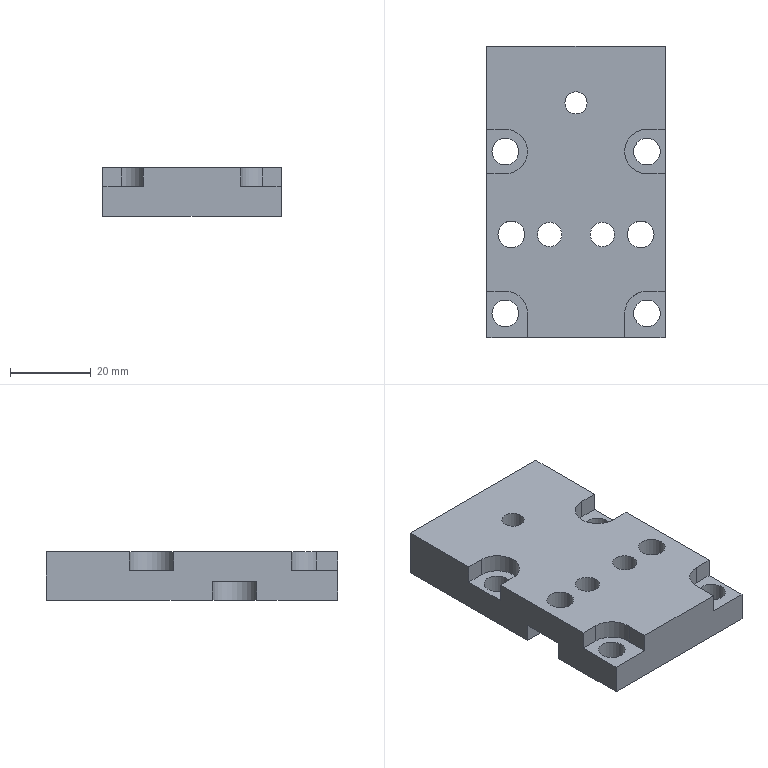Part | NX | features BREP 1 | 1 solid | 41 faces | box 44 x 72 x 12 mm | volume 32304 mm3 | plane 25 | cylinder 16 | commonest cylinder face diameters 6.6 x6 11 x6 6 x2 5.5 x1 10 x1
STEP:
#1=CARTESIAN_POINT('',(-22.,36.,0.));
#2=VERTEX_POINT('',#1);
#3=CARTESIAN_POINT('',(-22.,-5.,0.));
#4=VERTEX_POINT('',#3);
#5=CARTESIAN_POINT('',(-22.,0.,0.));
#6=DIRECTION('',(0.,-1.,0.));
#7=VECTOR('',#6,1000.);
#8=LINE('',#5,#7);
#9=EDGE_CURVE('',#2,#4,#8,.T.);
#10=ORIENTED_EDGE('',*,*,#9,.F.);
#11=CARTESIAN_POINT('',(22.,36.,0.));
#12=VERTEX_POINT('',#11);
#13=CARTESIAN_POINT('',(0.,36.,0.));
#14=DIRECTION('',(-1.,0.,0.));
#15=VECTOR('',#14,1000.);
#16=LINE('',#13,#15);
#17=EDGE_CURVE('',#12,#2,#16,.T.);
#18=ORIENTED_EDGE('',*,*,#17,.F.);
#19=CARTESIAN_POINT('',(22.,-5.,0.));
#20=VERTEX_POINT('',#19);
#21=CARTESIAN_POINT('',(22.,0.,0.));
#22=DIRECTION('',(0.,1.,0.));
#23=VECTOR('',#22,1000.);
#24=LINE('',#21,#23);
#25=EDGE_CURVE('',#20,#12,#24,.T.);
#26=ORIENTED_EDGE('',*,*,#25,.F.);
#27=CARTESIAN_POINT('',(16.,-5.,0.));
#28=VERTEX_POINT('',#27);
#29=CARTESIAN_POINT('',(0.,-5.,0.));
#30=DIRECTION('',(1.,0.,0.));
#31=VECTOR('',#30,1000.);
#32=LINE('',#29,#31);
#33=EDGE_CURVE('',#28,#20,#32,.T.);
#34=ORIENTED_EDGE('',*,*,#33,.F.);
#35=CARTESIAN_POINT('',(16.,-16.,0.));
#36=VERTEX_POINT('',#35);
#37=CARTESIAN_POINT('',(16.,-10.5,0.));
#38=DIRECTION('',(0.,0.,-1.));
#39=DIRECTION('',(-1.,0.,0.));
#40=AXIS2_PLACEMENT_3D('',#37,#38,#39);
#41=CIRCLE('',#40,5.5);
#42=EDGE_CURVE('',#36,#28,#41,.T.);
#43=ORIENTED_EDGE('',*,*,#42,.F.);
#44=CARTESIAN_POINT('',(22.,-16.,0.));
#45=VERTEX_POINT('',#44);
#46=CARTESIAN_POINT('',(0.,-16.,0.));
#47=DIRECTION('',(-1.,0.,0.));
#48=VECTOR('',#47,1000.);
#49=LINE('',#46,#48);
#50=EDGE_CURVE('',#45,#36,#49,.T.);
#51=ORIENTED_EDGE('',*,*,#50,.F.);
#52=CARTESIAN_POINT('',(22.,-36.,0.));
#53=VERTEX_POINT('',#52);
#54=CARTESIAN_POINT('',(22.,0.,0.));
#55=DIRECTION('',(0.,1.,0.));
#56=VECTOR('',#55,1000.);
#57=LINE('',#54,#56);
#58=EDGE_CURVE('',#53,#45,#57,.T.);
#59=ORIENTED_EDGE('',*,*,#58,.F.);
#60=CARTESIAN_POINT('',(-22.,-36.,0.));
#61=VERTEX_POINT('',#60);
#62=CARTESIAN_POINT('',(0.,-36.,0.));
#63=DIRECTION('',(1.,0.,0.));
#64=VECTOR('',#63,1000.);
#65=LINE('',#62,#64);
#66=EDGE_CURVE('',#61,#53,#65,.T.);
#67=ORIENTED_EDGE('',*,*,#66,.F.);
#68=CARTESIAN_POINT('',(-22.,-16.,0.));
#69=VERTEX_POINT('',#68);
#70=CARTESIAN_POINT('',(-22.,0.,0.));
#71=DIRECTION('',(0.,-1.,0.));
#72=VECTOR('',#71,1000.);
#73=LINE('',#70,#72);
#74=EDGE_CURVE('',#69,#61,#73,.T.);
#75=ORIENTED_EDGE('',*,*,#74,.F.);
#76=CARTESIAN_POINT('',(-16.,-16.,0.));
#77=VERTEX_POINT('',#76);
#78=CARTESIAN_POINT('',(0.,-16.,0.));
#79=DIRECTION('',(-1.,0.,0.));
#80=VECTOR('',#79,1000.);
#81=LINE('',#78,#80);
#82=EDGE_CURVE('',#77,#69,#81,.T.);
#83=ORIENTED_EDGE('',*,*,#82,.F.);
#84=CARTESIAN_POINT('',(-16.,-5.,0.));
#85=VERTEX_POINT('',#84);
#86=CARTESIAN_POINT('',(-16.,-10.5,0.));
#87=DIRECTION('',(0.,0.,-1.));
#88=DIRECTION('',(-1.,0.,0.));
#89=AXIS2_PLACEMENT_3D('',#86,#87,#88);
#90=CIRCLE('',#89,5.5);
#91=EDGE_CURVE('',#85,#77,#90,.T.);
#92=ORIENTED_EDGE('',*,*,#91,.F.);
#93=CARTESIAN_POINT('',(0.,-5.,0.));
#94=DIRECTION('',(1.,0.,0.));
#95=VECTOR('',#94,1000.);
#96=LINE('',#93,#95);
#97=EDGE_CURVE('',#4,#85,#96,.T.);
#98=ORIENTED_EDGE('',*,*,#97,.F.);
#99=EDGE_LOOP('',(#10,#18,#26,#34,#43,#51,#59,#67,#75,#83,#92,#98));
#100=FACE_BOUND('',#99,.T.);
#101=CARTESIAN_POINT('',(-3.5,-10.5,0.));
#102=VERTEX_POINT('',#101);
#103=CARTESIAN_POINT('',(-6.5,-10.5,0.));
#104=DIRECTION('',(0.,0.,-1.));
#105=DIRECTION('',(1.,0.,0.));
#106=AXIS2_PLACEMENT_3D('',#103,#104,#105);
#107=CIRCLE('',#106,3.);
#108=EDGE_CURVE('',#102,#102,#107,.T.);
#109=ORIENTED_EDGE('',*,*,#108,.F.);
#110=EDGE_LOOP('',(#109));
#111=FACE_BOUND('',#110,.T.);
#112=CARTESIAN_POINT('',(9.5,-10.5,0.));
#113=VERTEX_POINT('',#112);
#114=CARTESIAN_POINT('',(6.5,-10.5,0.));
#115=DIRECTION('',(0.,0.,-1.));
#116=DIRECTION('',(1.,0.,0.));
#117=AXIS2_PLACEMENT_3D('',#114,#115,#116);
#118=CIRCLE('',#117,3.);
#119=EDGE_CURVE('',#113,#113,#118,.T.);
#120=ORIENTED_EDGE('',*,*,#119,.F.);
#121=EDGE_LOOP('',(#120));
#122=FACE_BOUND('',#121,.T.);
#123=CARTESIAN_POINT('',(20.825,-30.,0.));
#124=VERTEX_POINT('',#123);
#125=CARTESIAN_POINT('',(17.525,-30.,0.));
#126=DIRECTION('',(0.,0.,-1.));
#127=DIRECTION('',(1.,0.,0.));
#128=AXIS2_PLACEMENT_3D('',#125,#126,#127);
#129=CIRCLE('',#128,3.3);
#130=EDGE_CURVE('',#124,#124,#129,.T.);
#131=ORIENTED_EDGE('',*,*,#130,.F.);
#132=EDGE_LOOP('',(#131));
#133=FACE_BOUND('',#132,.T.);
#134=CARTESIAN_POINT('',(-14.175,-30.,0.));
#135=VERTEX_POINT('',#134);
#136=CARTESIAN_POINT('',(-17.475,-30.,0.));
#137=DIRECTION('',(0.,0.,-1.));
#138=DIRECTION('',(1.,0.,0.));
#139=AXIS2_PLACEMENT_3D('',#136,#137,#138);
#140=CIRCLE('',#139,3.3);
#141=EDGE_CURVE('',#135,#135,#140,.T.);
#142=ORIENTED_EDGE('',*,*,#141,.F.);
#143=EDGE_LOOP('',(#142));
#144=FACE_BOUND('',#143,.T.);
#145=CARTESIAN_POINT('',(-14.175,10.,0.));
#146=VERTEX_POINT('',#145);
#147=CARTESIAN_POINT('',(-17.475,10.,0.));
#148=DIRECTION('',(0.,0.,-1.));
#149=DIRECTION('',(1.,0.,0.));
#150=AXIS2_PLACEMENT_3D('',#147,#148,#149);
#151=CIRCLE('',#150,3.3);
#152=EDGE_CURVE('',#146,#146,#151,.T.);
#153=ORIENTED_EDGE('',*,*,#152,.F.);
#154=EDGE_LOOP('',(#153));
#155=FACE_BOUND('',#154,.T.);
#156=CARTESIAN_POINT('',(20.825,10.,0.));
#157=VERTEX_POINT('',#156);
#158=CARTESIAN_POINT('',(17.525,10.,0.));
#159=DIRECTION('',(0.,0.,-1.));
#160=DIRECTION('',(1.,0.,0.));
#161=AXIS2_PLACEMENT_3D('',#158,#159,#160);
#162=CIRCLE('',#161,3.3);
#163=EDGE_CURVE('',#157,#157,#162,.T.);
#164=ORIENTED_EDGE('',*,*,#163,.F.);
#165=EDGE_LOOP('',(#164));
#166=FACE_BOUND('',#165,.T.);
#167=CARTESIAN_POINT('',(-5.,22.,0.));
#168=VERTEX_POINT('',#167);
#169=CARTESIAN_POINT('',(0.,22.,0.));
#170=DIRECTION('',(0.,0.,-1.));
#171=DIRECTION('',(-1.,0.,0.));
#172=AXIS2_PLACEMENT_3D('',#169,#170,#171);
#173=CIRCLE('',#172,5.);
#174=EDGE_CURVE('',#168,#168,#173,.T.);
#175=ORIENTED_EDGE('',*,*,#174,.F.);
#176=EDGE_LOOP('',(#175));
#177=FACE_BOUND('',#176,.T.);
#178=CARTESIAN_POINT('',(0.,0.,0.));
#179=DIRECTION('',(0.,0.,1.));
#180=DIRECTION('',(-1.,0.,0.));
#181=AXIS2_PLACEMENT_3D('',#178,#179,#180);
#182=PLANE('',#181);
#183=ADVANCED_FACE('',(#100,#111,#122,#133,#144,#155,#166,#177),#182,.F.);
#184=ORIENTED_EDGE('',*,*,#97,.T.);
#185=CARTESIAN_POINT('',(-16.,-5.,4.6));
#186=VERTEX_POINT('',#185);
#187=CARTESIAN_POINT('',(-16.,-5.,17.13));
#188=DIRECTION('',(0.,0.,1.));
#189=VECTOR('',#188,1000.);
#190=LINE('',#187,#189);
#191=EDGE_CURVE('',#85,#186,#190,.T.);
#192=ORIENTED_EDGE('',*,*,#191,.T.);
#193=CARTESIAN_POINT('',(-22.,-5.,4.6));
#194=VERTEX_POINT('',#193);
#195=CARTESIAN_POINT('',(-16.,-5.,4.6));
#196=DIRECTION('',(-1.,0.,0.));
#197=VECTOR('',#196,1000.);
#198=LINE('',#195,#197);
#199=EDGE_CURVE('',#186,#194,#198,.T.);
#200=ORIENTED_EDGE('',*,*,#199,.T.);
#201=CARTESIAN_POINT('',(-22.,-5.,17.13));
#202=DIRECTION('',(0.,0.,-1.));
#203=VECTOR('',#202,1000.);
#204=LINE('',#201,#203);
#205=EDGE_CURVE('',#194,#4,#204,.T.);
#206=ORIENTED_EDGE('',*,*,#205,.T.);
#207=EDGE_LOOP('',(#184,#192,#200,#206));
#208=FACE_BOUND('',#207,.T.);
#209=CARTESIAN_POINT('',(-16.,-5.,17.13));
#210=DIRECTION('',(0.,-1.,0.));
#211=DIRECTION('',(-1.,0.,0.));
#212=AXIS2_PLACEMENT_3D('',#209,#210,#211);
#213=PLANE('',#212);
#214=ADVANCED_FACE('',(#208),#213,.T.);
#215=CARTESIAN_POINT('',(-22.,-16.,4.6));
#216=VERTEX_POINT('',#215);
#217=CARTESIAN_POINT('',(-22.,36.,4.6));
#218=DIRECTION('',(0.,1.,0.));
#219=VECTOR('',#218,1000.);
#220=LINE('',#217,#219);
#221=EDGE_CURVE('',#216,#194,#220,.T.);
#222=ORIENTED_EDGE('',*,*,#221,.F.);
#223=CARTESIAN_POINT('',(-22.,-16.,12.));
#224=DIRECTION('',(0.,0.,1.));
#225=VECTOR('',#224,1000.);
#226=LINE('',#223,#225);
#227=EDGE_CURVE('',#69,#216,#226,.T.);
#228=ORIENTED_EDGE('',*,*,#227,.F.);
#229=ORIENTED_EDGE('',*,*,#74,.T.);
#230=CARTESIAN_POINT('',(-22.,-36.,7.4));
#231=VERTEX_POINT('',#230);
#232=CARTESIAN_POINT('',(-22.,-36.,12.));
#233=DIRECTION('',(0.,0.,-1.));
#234=VECTOR('',#233,1000.);
#235=LINE('',#232,#234);
#236=EDGE_CURVE('',#231,#61,#235,.T.);
#237=ORIENTED_EDGE('',*,*,#236,.F.);
#238=CARTESIAN_POINT('',(-22.,-24.5,7.4));
#239=VERTEX_POINT('',#238);
#240=CARTESIAN_POINT('',(-22.,36.,7.4));
#241=DIRECTION('',(0.,-1.,0.));
#242=VECTOR('',#241,1000.);
#243=LINE('',#240,#242);
#244=EDGE_CURVE('',#239,#231,#243,.T.);
#245=ORIENTED_EDGE('',*,*,#244,.F.);
#246=CARTESIAN_POINT('',(-22.,-24.5,12.));
#247=VERTEX_POINT('',#246);
#248=CARTESIAN_POINT('',(-22.,-24.5,12.));
#249=DIRECTION('',(0.,0.,-1.));
#250=VECTOR('',#249,1000.);
#251=LINE('',#248,#250);
#252=EDGE_CURVE('',#247,#239,#251,.T.);
#253=ORIENTED_EDGE('',*,*,#252,.F.);
#254=CARTESIAN_POINT('',(-22.,4.5,12.));
#255=VERTEX_POINT('',#254);
#256=CARTESIAN_POINT('',(-22.,36.,12.));
#257=DIRECTION('',(0.,-1.,0.));
#258=VECTOR('',#257,1000.);
#259=LINE('',#256,#258);
#260=EDGE_CURVE('',#255,#247,#259,.T.);
#261=ORIENTED_EDGE('',*,*,#260,.F.);
#262=CARTESIAN_POINT('',(-22.,4.5,7.4));
#263=VERTEX_POINT('',#262);
#264=CARTESIAN_POINT('',(-22.,4.5,12.));
#265=DIRECTION('',(0.,0.,1.));
#266=VECTOR('',#265,1000.);
#267=LINE('',#264,#266);
#268=EDGE_CURVE('',#263,#255,#267,.T.);
#269=ORIENTED_EDGE('',*,*,#268,.F.);
#270=CARTESIAN_POINT('',(-22.,15.5,7.4));
#271=VERTEX_POINT('',#270);
#272=CARTESIAN_POINT('',(-22.,36.,7.4));
#273=DIRECTION('',(0.,-1.,0.));
#274=VECTOR('',#273,1000.);
#275=LINE('',#272,#274);
#276=EDGE_CURVE('',#271,#263,#275,.T.);
#277=ORIENTED_EDGE('',*,*,#276,.F.);
#278=CARTESIAN_POINT('',(-22.,15.5,12.));
#279=VERTEX_POINT('',#278);
#280=CARTESIAN_POINT('',(-22.,15.5,12.));
#281=DIRECTION('',(0.,0.,-1.));
#282=VECTOR('',#281,1000.);
#283=LINE('',#280,#282);
#284=EDGE_CURVE('',#279,#271,#283,.T.);
#285=ORIENTED_EDGE('',*,*,#284,.F.);
#286=CARTESIAN_POINT('',(-22.,36.,12.));
#287=VERTEX_POINT('',#286);
#288=CARTESIAN_POINT('',(-22.,36.,12.));
#289=DIRECTION('',(0.,-1.,0.));
#290=VECTOR('',#289,1000.);
#291=LINE('',#288,#290);
#292=EDGE_CURVE('',#287,#279,#291,.T.);
#293=ORIENTED_EDGE('',*,*,#292,.F.);
#294=CARTESIAN_POINT('',(-22.,36.,12.));
#295=DIRECTION('',(0.,0.,1.));
#296=VECTOR('',#295,1000.);
#297=LINE('',#294,#296);
#298=EDGE_CURVE('',#2,#287,#297,.T.);
#299=ORIENTED_EDGE('',*,*,#298,.F.);
#300=ORIENTED_EDGE('',*,*,#9,.T.);
#301=ORIENTED_EDGE('',*,*,#205,.F.);
#302=EDGE_LOOP('',(#222,#228,#229,#237,#245,#253,#261,#269,#277,#285,#293,#299,#300,#301));
#303=FACE_BOUND('',#302,.T.);
#304=CARTESIAN_POINT('',(-22.,36.,12.));
#305=DIRECTION('',(1.,0.,0.));
#306=DIRECTION('',(0.,-1.,0.));
#307=AXIS2_PLACEMENT_3D('',#304,#305,#306);
#308=PLANE('',#307);
#309=ADVANCED_FACE('',(#303),#308,.F.);
#310=ORIENTED_EDGE('',*,*,#298,.T.);
#311=CARTESIAN_POINT('',(22.,36.,12.));
#312=VERTEX_POINT('',#311);
#313=CARTESIAN_POINT('',(-22.,36.,12.));
#314=DIRECTION('',(-1.,0.,0.));
#315=VECTOR('',#314,1000.);
#316=LINE('',#313,#315);
#317=EDGE_CURVE('',#312,#287,#316,.T.);
#318=ORIENTED_EDGE('',*,*,#317,.F.);
#319=CARTESIAN_POINT('',(22.,36.,12.));
#320=DIRECTION('',(0.,0.,1.));
#321=VECTOR('',#320,1000.);
#322=LINE('',#319,#321);
#323=EDGE_CURVE('',#12,#312,#322,.T.);
#324=ORIENTED_EDGE('',*,*,#323,.F.);
#325=ORIENTED_EDGE('',*,*,#17,.T.);
#326=EDGE_LOOP('',(#310,#318,#324,#325));
#327=FACE_BOUND('',#326,.T.);
#328=CARTESIAN_POINT('',(-22.,36.,12.));
#329=DIRECTION('',(0.,-1.,0.));
#330=DIRECTION('',(0.,0.,1.));
#331=AXIS2_PLACEMENT_3D('',#328,#329,#330);
#332=PLANE('',#331);
#333=ADVANCED_FACE('',(#327),#332,.F.);
#334=CARTESIAN_POINT('',(22.,-5.,4.6));
#335=VERTEX_POINT('',#334);
#336=CARTESIAN_POINT('',(22.,-5.,12.));
#337=DIRECTION('',(0.,0.,1.));
#338=VECTOR('',#337,1000.);
#339=LINE('',#336,#338);
#340=EDGE_CURVE('',#20,#335,#339,.T.);
#341=ORIENTED_EDGE('',*,*,#340,.F.);
#342=ORIENTED_EDGE('',*,*,#25,.T.);
#343=ORIENTED_EDGE('',*,*,#323,.T.);
#344=CARTESIAN_POINT('',(22.,15.5,12.));
#345=VERTEX_POINT('',#344);
#346=CARTESIAN_POINT('',(22.,36.,12.));
#347=DIRECTION('',(0.,1.,0.));
#348=VECTOR('',#347,1000.);
#349=LINE('',#346,#348);
#350=EDGE_CURVE('',#345,#312,#349,.T.);
#351=ORIENTED_EDGE('',*,*,#350,.F.);
#352=CARTESIAN_POINT('',(22.,15.5,7.4));
#353=VERTEX_POINT('',#352);
#354=CARTESIAN_POINT('',(22.,15.5,12.));
#355=DIRECTION('',(0.,0.,1.));
#356=VECTOR('',#355,1000.);
#357=LINE('',#354,#356);
#358=EDGE_CURVE('',#353,#345,#357,.T.);
#359=ORIENTED_EDGE('',*,*,#358,.F.);
#360=CARTESIAN_POINT('',(22.,4.5,7.4));
#361=VERTEX_POINT('',#360);
#362=CARTESIAN_POINT('',(22.,36.,7.4));
#363=DIRECTION('',(0.,1.,0.));
#364=VECTOR('',#363,1000.);
#365=LINE('',#362,#364);
#366=EDGE_CURVE('',#361,#353,#365,.T.);
#367=ORIENTED_EDGE('',*,*,#366,.F.);
#368=CARTESIAN_POINT('',(22.,4.5,12.));
#369=VERTEX_POINT('',#368);
#370=CARTESIAN_POINT('',(22.,4.5,12.));
#371=DIRECTION('',(0.,0.,-1.));
#372=VECTOR('',#371,1000.);
#373=LINE('',#370,#372);
#374=EDGE_CURVE('',#369,#361,#373,.T.);
#375=ORIENTED_EDGE('',*,*,#374,.F.);
#376=CARTESIAN_POINT('',(22.,-24.5,12.));
#377=VERTEX_POINT('',#376);
#378=CARTESIAN_POINT('',(22.,36.,12.));
#379=DIRECTION('',(0.,1.,0.));
#380=VECTOR('',#379,1000.);
#381=LINE('',#378,#380);
#382=EDGE_CURVE('',#377,#369,#381,.T.);
#383=ORIENTED_EDGE('',*,*,#382,.F.);
#384=CARTESIAN_POINT('',(22.,-24.5,7.4));
#385=VERTEX_POINT('',#384);
#386=CARTESIAN_POINT('',(22.,-24.5,12.));
#387=DIRECTION('',(0.,0.,1.));
#388=VECTOR('',#387,1000.);
#389=LINE('',#386,#388);
#390=EDGE_CURVE('',#385,#377,#389,.T.);
#391=ORIENTED_EDGE('',*,*,#390,.F.);
#392=CARTESIAN_POINT('',(22.,-36.,7.4));
#393=VERTEX_POINT('',#392);
#394=CARTESIAN_POINT('',(22.,36.,7.4));
#395=DIRECTION('',(0.,1.,0.));
#396=VECTOR('',#395,1000.);
#397=LINE('',#394,#396);
#398=EDGE_CURVE('',#393,#385,#397,.T.);
#399=ORIENTED_EDGE('',*,*,#398,.F.);
#400=CARTESIAN_POINT('',(22.,-36.,12.));
#401=DIRECTION('',(0.,0.,1.));
#402=VECTOR('',#401,1000.);
#403=LINE('',#400,#402);
#404=EDGE_CURVE('',#53,#393,#403,.T.);
#405=ORIENTED_EDGE('',*,*,#404,.F.);
#406=ORIENTED_EDGE('',*,*,#58,.T.);
#407=CARTESIAN_POINT('',(22.,-16.,4.6));
#408=VERTEX_POINT('',#407);
#409=CARTESIAN_POINT('',(22.,-16.,12.));
#410=DIRECTION('',(0.,0.,-1.));
#411=VECTOR('',#410,1000.);
#412=LINE('',#409,#411);
#413=EDGE_CURVE('',#408,#45,#412,.T.);
#414=ORIENTED_EDGE('',*,*,#413,.F.);
#415=CARTESIAN_POINT('',(22.,36.,4.6));
#416=DIRECTION('',(0.,-1.,0.));
#417=VECTOR('',#416,1000.);
#418=LINE('',#415,#417);
#419=EDGE_CURVE('',#335,#408,#418,.T.);
#420=ORIENTED_EDGE('',*,*,#419,.F.);
#421=EDGE_LOOP('',(#341,#342,#343,#351,#359,#367,#375,#383,#391,#399,#405,#406,#414,#420));
#422=FACE_BOUND('',#421,.T.);
#423=CARTESIAN_POINT('',(22.,36.,12.));
#424=DIRECTION('',(-1.,0.,0.));
#425=DIRECTION('',(0.,1.,0.));
#426=AXIS2_PLACEMENT_3D('',#423,#424,#425);
#427=PLANE('',#426);
#428=ADVANCED_FACE('',(#422),#427,.F.);
#429=ORIENTED_EDGE('',*,*,#33,.T.);
#430=ORIENTED_EDGE('',*,*,#340,.T.);
#431=CARTESIAN_POINT('',(16.,-5.,4.6));
#432=VERTEX_POINT('',#431);
#433=CARTESIAN_POINT('',(16.,-5.,4.6));
#434=DIRECTION('',(1.,0.,0.));
#435=VECTOR('',#434,1000.);
#436=LINE('',#433,#435);
#437=EDGE_CURVE('',#432,#335,#436,.T.);
#438=ORIENTED_EDGE('',*,*,#437,.F.);
#439=CARTESIAN_POINT('',(16.,-5.,17.13));
#440=DIRECTION('',(0.,0.,1.));
#441=VECTOR('',#440,1000.);
#442=LINE('',#439,#441);
#443=EDGE_CURVE('',#28,#432,#442,.T.);
#444=ORIENTED_EDGE('',*,*,#443,.F.);
#445=EDGE_LOOP('',(#429,#430,#438,#444));
#446=FACE_BOUND('',#445,.T.);
#447=CARTESIAN_POINT('',(16.,-5.,17.13));
#448=DIRECTION('',(0.,1.,0.));
#449=DIRECTION('',(1.,0.,0.));
#450=AXIS2_PLACEMENT_3D('',#447,#448,#449);
#451=PLANE('',#450);
#452=ADVANCED_FACE('',(#446),#451,.F.);
#453=CARTESIAN_POINT('',(16.,-16.,4.6));
#454=VERTEX_POINT('',#453);
#455=CARTESIAN_POINT('',(16.,-10.5,4.6));
#456=DIRECTION('',(0.,0.,-1.));
#457=DIRECTION('',(-1.,0.,0.));
#458=AXIS2_PLACEMENT_3D('',#455,#456,#457);
#459=CIRCLE('',#458,5.5);
#460=EDGE_CURVE('',#454,#432,#459,.T.);
#461=ORIENTED_EDGE('',*,*,#460,.F.);
#462=CARTESIAN_POINT('',(16.,-16.,0.));
#463=DIRECTION('',(0.,0.,1.));
#464=VECTOR('',#463,1000.);
#465=LINE('',#462,#464);
#466=EDGE_CURVE('',#36,#454,#465,.T.);
#467=ORIENTED_EDGE('',*,*,#466,.F.);
#468=ORIENTED_EDGE('',*,*,#42,.T.);
#469=ORIENTED_EDGE('',*,*,#443,.T.);
#470=EDGE_LOOP('',(#461,#467,#468,#469));
#471=FACE_BOUND('',#470,.T.);
#472=CARTESIAN_POINT('',(16.,-10.5,0.));
#473=DIRECTION('',(0.,0.,-1.));
#474=DIRECTION('',(1.,0.,0.));
#475=AXIS2_PLACEMENT_3D('',#472,#473,#474);
#476=CYLINDRICAL_SURFACE('',#475,5.5);
#477=ADVANCED_FACE('',(#471),#476,.F.);
#478=ORIENTED_EDGE('',*,*,#50,.T.);
#479=ORIENTED_EDGE('',*,*,#466,.T.);
#480=CARTESIAN_POINT('',(22.,-16.,4.6));
#481=DIRECTION('',(-1.,0.,0.));
#482=VECTOR('',#481,1000.);
#483=LINE('',#480,#482);
#484=EDGE_CURVE('',#408,#454,#483,.T.);
#485=ORIENTED_EDGE('',*,*,#484,.F.);
#486=ORIENTED_EDGE('',*,*,#413,.T.);
#487=EDGE_LOOP('',(#478,#479,#485,#486));
#488=FACE_BOUND('',#487,.T.);
#489=CARTESIAN_POINT('',(22.,-16.,17.13));
#490=DIRECTION('',(0.,-1.,0.));
#491=DIRECTION('',(-1.,0.,0.));
#492=AXIS2_PLACEMENT_3D('',#489,#490,#491);
#493=PLANE('',#492);
#494=ADVANCED_FACE('',(#488),#493,.F.);
#495=CARTESIAN_POINT('',(-12.025,-36.,7.4));
#496=VERTEX_POINT('',#495);
#497=CARTESIAN_POINT('',(-22.,-36.,7.4));
#498=DIRECTION('',(1.,0.,0.));
#499=VECTOR('',#498,1000.);
#500=LINE('',#497,#499);
#501=EDGE_CURVE('',#231,#496,#500,.T.);
#502=ORIENTED_EDGE('',*,*,#501,.F.);
#503=ORIENTED_EDGE('',*,*,#236,.T.);
#504=ORIENTED_EDGE('',*,*,#66,.T.);
#505=ORIENTED_EDGE('',*,*,#404,.T.);
#506=CARTESIAN_POINT('',(12.025,-36.,7.4));
#507=VERTEX_POINT('',#506);
#508=CARTESIAN_POINT('',(-22.,-36.,7.4));
#509=DIRECTION('',(1.,0.,0.));
#510=VECTOR('',#509,1000.);
#511=LINE('',#508,#510);
#512=EDGE_CURVE('',#507,#393,#511,.T.);
#513=ORIENTED_EDGE('',*,*,#512,.F.);
#514=CARTESIAN_POINT('',(12.025,-36.,12.));
#515=VERTEX_POINT('',#514);
#516=CARTESIAN_POINT('',(12.025,-36.,12.));
#517=DIRECTION('',(0.,0.,-1.));
#518=VECTOR('',#517,1000.);
#519=LINE('',#516,#518);
#520=EDGE_CURVE('',#515,#507,#519,.T.);
#521=ORIENTED_EDGE('',*,*,#520,.F.);
#522=CARTESIAN_POINT('',(-12.025,-36.,12.));
#523=VERTEX_POINT('',#522);
#524=CARTESIAN_POINT('',(-22.,-36.,12.));
#525=DIRECTION('',(1.,0.,0.));
#526=VECTOR('',#525,1000.);
#527=LINE('',#524,#526);
#528=EDGE_CURVE('',#523,#515,#527,.T.);
#529=ORIENTED_EDGE('',*,*,#528,.F.);
#530=CARTESIAN_POINT('',(-12.025,-36.,12.));
#531=DIRECTION('',(0.,0.,1.));
#532=VECTOR('',#531,1000.);
#533=LINE('',#530,#532);
#534=EDGE_CURVE('',#496,#523,#533,.T.);
#535=ORIENTED_EDGE('',*,*,#534,.F.);
#536=EDGE_LOOP('',(#502,#503,#504,#505,#513,#521,#529,#535));
#537=FACE_BOUND('',#536,.T.);
#538=CARTESIAN_POINT('',(-22.,-36.,12.));
#539=DIRECTION('',(0.,1.,0.));
#540=DIRECTION('',(0.,0.,-1.));
#541=AXIS2_PLACEMENT_3D('',#538,#539,#540);
#542=PLANE('',#541);
#543=ADVANCED_FACE('',(#537),#542,.F.);
#544=ORIENTED_EDGE('',*,*,#82,.T.);
#545=ORIENTED_EDGE('',*,*,#227,.T.);
#546=CARTESIAN_POINT('',(-16.,-16.,4.6));
#547=VERTEX_POINT('',#546);
#548=CARTESIAN_POINT('',(-22.,-16.,4.6));
#549=DIRECTION('',(1.,0.,0.));
#550=VECTOR('',#549,1000.);
#551=LINE('',#548,#550);
#552=EDGE_CURVE('',#216,#547,#551,.T.);
#553=ORIENTED_EDGE('',*,*,#552,.T.);
#554=CARTESIAN_POINT('',(-16.,-16.,17.13));
#555=DIRECTION('',(0.,0.,-1.));
#556=VECTOR('',#555,1000.);
#557=LINE('',#554,#556);
#558=EDGE_CURVE('',#547,#77,#557,.T.);
#559=ORIENTED_EDGE('',*,*,#558,.T.);
#560=EDGE_LOOP('',(#544,#545,#553,#559));
#561=FACE_BOUND('',#560,.T.);
#562=CARTESIAN_POINT('',(-22.,-16.,17.13));
#563=DIRECTION('',(0.,1.,0.));
#564=DIRECTION('',(1.,0.,0.));
#565=AXIS2_PLACEMENT_3D('',#562,#563,#564);
#566=PLANE('',#565);
#567=ADVANCED_FACE('',(#561),#566,.T.);
#568=ORIENTED_EDGE('',*,*,#91,.T.);
#569=ORIENTED_EDGE('',*,*,#558,.F.);
#570=CARTESIAN_POINT('',(-16.,-10.5,4.6));
#571=DIRECTION('',(0.,0.,-1.));
#572=DIRECTION('',(-1.,0.,0.));
#573=AXIS2_PLACEMENT_3D('',#570,#571,#572);
#574=CIRCLE('',#573,5.5);
#575=EDGE_CURVE('',#186,#547,#574,.T.);
#576=ORIENTED_EDGE('',*,*,#575,.F.);
#577=ORIENTED_EDGE('',*,*,#191,.F.);
#578=EDGE_LOOP('',(#568,#569,#576,#577));
#579=FACE_BOUND('',#578,.T.);
#580=CARTESIAN_POINT('',(-16.,-10.5,0.));
#581=DIRECTION('',(0.,0.,-1.));
#582=DIRECTION('',(1.,0.,0.));
#583=AXIS2_PLACEMENT_3D('',#580,#581,#582);
#584=CYLINDRICAL_SURFACE('',#583,5.5);
#585=ADVANCED_FACE('',(#579),#584,.F.);
#586=ORIENTED_EDGE('',*,*,#108,.T.);
#587=EDGE_LOOP('',(#586));
#588=FACE_BOUND('',#587,.T.);
#589=CARTESIAN_POINT('',(-3.5,-10.5,12.));
#590=VERTEX_POINT('',#589);
#591=CARTESIAN_POINT('',(-6.5,-10.5,12.));
#592=DIRECTION('',(0.,0.,-1.));
#593=DIRECTION('',(1.,0.,0.));
#594=AXIS2_PLACEMENT_3D('',#591,#592,#593);
#595=CIRCLE('',#594,3.);
#596=EDGE_CURVE('',#590,#590,#595,.T.);
#597=ORIENTED_EDGE('',*,*,#596,.F.);
#598=EDGE_LOOP('',(#597));
#599=FACE_BOUND('',#598,.T.);
#600=CARTESIAN_POINT('',(-6.5,-10.5,12.));
#601=DIRECTION('',(0.,0.,1.));
#602=DIRECTION('',(-1.,0.,0.));
#603=AXIS2_PLACEMENT_3D('',#600,#601,#602);
#604=CYLINDRICAL_SURFACE('',#603,3.);
#605=ADVANCED_FACE('',(#588,#599),#604,.F.);
#606=ORIENTED_EDGE('',*,*,#119,.T.);
#607=EDGE_LOOP('',(#606));
#608=FACE_BOUND('',#607,.T.);
#609=CARTESIAN_POINT('',(9.5,-10.5,12.));
#610=VERTEX_POINT('',#609);
#611=CARTESIAN_POINT('',(6.5,-10.5,12.));
#612=DIRECTION('',(0.,0.,-1.));
#613=DIRECTION('',(1.,0.,0.));
#614=AXIS2_PLACEMENT_3D('',#611,#612,#613);
#615=CIRCLE('',#614,3.);
#616=EDGE_CURVE('',#610,#610,#615,.T.);
#617=ORIENTED_EDGE('',*,*,#616,.F.);
#618=EDGE_LOOP('',(#617));
#619=FACE_BOUND('',#618,.T.);
#620=CARTESIAN_POINT('',(6.5,-10.5,12.));
#621=DIRECTION('',(0.,0.,1.));
#622=DIRECTION('',(-1.,0.,0.));
#623=AXIS2_PLACEMENT_3D('',#620,#621,#622);
#624=CYLINDRICAL_SURFACE('',#623,3.);
#625=ADVANCED_FACE('',(#608,#619),#624,.F.);
#626=ORIENTED_EDGE('',*,*,#130,.T.);
#627=EDGE_LOOP('',(#626));
#628=FACE_BOUND('',#627,.T.);
#629=CARTESIAN_POINT('',(20.825,-30.,7.4));
#630=VERTEX_POINT('',#629);
#631=CARTESIAN_POINT('',(17.525,-30.,7.4));
#632=DIRECTION('',(0.,0.,-1.));
#633=DIRECTION('',(1.,0.,0.));
#634=AXIS2_PLACEMENT_3D('',#631,#632,#633);
#635=CIRCLE('',#634,3.3);
#636=EDGE_CURVE('',#630,#630,#635,.T.);
#637=ORIENTED_EDGE('',*,*,#636,.F.);
#638=EDGE_LOOP('',(#637));
#639=FACE_BOUND('',#638,.T.);
#640=CARTESIAN_POINT('',(17.525,-30.,12.));
#641=DIRECTION('',(0.,0.,1.));
#642=DIRECTION('',(-1.,0.,0.));
#643=AXIS2_PLACEMENT_3D('',#640,#641,#642);
#644=CYLINDRICAL_SURFACE('',#643,3.3);
#645=ADVANCED_FACE('',(#628,#639),#644,.F.);
#646=ORIENTED_EDGE('',*,*,#141,.T.);
#647=EDGE_LOOP('',(#646));
#648=FACE_BOUND('',#647,.T.);
#649=CARTESIAN_POINT('',(-14.175,-30.,7.4));
#650=VERTEX_POINT('',#649);
#651=CARTESIAN_POINT('',(-17.475,-30.,7.4));
#652=DIRECTION('',(0.,0.,-1.));
#653=DIRECTION('',(1.,0.,0.));
#654=AXIS2_PLACEMENT_3D('',#651,#652,#653);
#655=CIRCLE('',#654,3.3);
#656=EDGE_CURVE('',#650,#650,#655,.T.);
#657=ORIENTED_EDGE('',*,*,#656,.F.);
#658=EDGE_LOOP('',(#657));
#659=FACE_BOUND('',#658,.T.);
#660=CARTESIAN_POINT('',(-17.475,-30.,12.));
#661=DIRECTION('',(0.,0.,1.));
#662=DIRECTION('',(-1.,0.,0.));
#663=AXIS2_PLACEMENT_3D('',#660,#661,#662);
#664=CYLINDRICAL_SURFACE('',#663,3.3);
#665=ADVANCED_FACE('',(#648,#659),#664,.F.);
#666=ORIENTED_EDGE('',*,*,#152,.T.);
#667=EDGE_LOOP('',(#666));
#668=FACE_BOUND('',#667,.T.);
#669=CARTESIAN_POINT('',(-14.175,10.,7.4));
#670=VERTEX_POINT('',#669);
#671=CARTESIAN_POINT('',(-17.475,10.,7.4));
#672=DIRECTION('',(0.,0.,-1.));
#673=DIRECTION('',(1.,0.,0.));
#674=AXIS2_PLACEMENT_3D('',#671,#672,#673);
#675=CIRCLE('',#674,3.3);
#676=EDGE_CURVE('',#670,#670,#675,.T.);
#677=ORIENTED_EDGE('',*,*,#676,.F.);
#678=EDGE_LOOP('',(#677));
#679=FACE_BOUND('',#678,.T.);
#680=CARTESIAN_POINT('',(-17.475,10.,12.));
#681=DIRECTION('',(0.,0.,1.));
#682=DIRECTION('',(-1.,0.,0.));
#683=AXIS2_PLACEMENT_3D('',#680,#681,#682);
#684=CYLINDRICAL_SURFACE('',#683,3.3);
#685=ADVANCED_FACE('',(#668,#679),#684,.F.);
#686=ORIENTED_EDGE('',*,*,#163,.T.);
#687=EDGE_LOOP('',(#686));
#688=FACE_BOUND('',#687,.T.);
#689=CARTESIAN_POINT('',(20.825,10.,7.4));
#690=VERTEX_POINT('',#689);
#691=CARTESIAN_POINT('',(17.525,10.,7.4));
#692=DIRECTION('',(0.,0.,-1.));
#693=DIRECTION('',(1.,0.,0.));
#694=AXIS2_PLACEMENT_3D('',#691,#692,#693);
#695=CIRCLE('',#694,3.3);
#696=EDGE_CURVE('',#690,#690,#695,.T.);
#697=ORIENTED_EDGE('',*,*,#696,.F.);
#698=EDGE_LOOP('',(#697));
#699=FACE_BOUND('',#698,.T.);
#700=CARTESIAN_POINT('',(17.525,10.,12.));
#701=DIRECTION('',(0.,0.,1.));
#702=DIRECTION('',(-1.,0.,0.));
#703=AXIS2_PLACEMENT_3D('',#700,#701,#702);
#704=CYLINDRICAL_SURFACE('',#703,3.3);
#705=ADVANCED_FACE('',(#688,#699),#704,.F.);
#706=CARTESIAN_POINT('',(-5.,22.,5.4));
#707=VERTEX_POINT('',#706);
#708=CARTESIAN_POINT('',(0.,22.,5.4));
#709=DIRECTION('',(0.,0.,-1.));
#710=DIRECTION('',(-1.,0.,0.));
#711=AXIS2_PLACEMENT_3D('',#708,#709,#710);
#712=CIRCLE('',#711,5.);
#713=EDGE_CURVE('',#707,#707,#712,.T.);
#714=ORIENTED_EDGE('',*,*,#713,.F.);
#715=EDGE_LOOP('',(#714));
#716=FACE_BOUND('',#715,.T.);
#717=ORIENTED_EDGE('',*,*,#174,.T.);
#718=EDGE_LOOP('',(#717));
#719=FACE_BOUND('',#718,.T.);
#720=CARTESIAN_POINT('',(0.,22.,0.));
#721=DIRECTION('',(0.,0.,-1.));
#722=DIRECTION('',(1.,0.,0.));
#723=AXIS2_PLACEMENT_3D('',#720,#721,#722);
#724=CYLINDRICAL_SURFACE('',#723,5.);
#725=ADVANCED_FACE('',(#716,#719),#724,.F.);
#726=ORIENTED_EDGE('',*,*,#575,.T.);
#727=ORIENTED_EDGE('',*,*,#552,.F.);
#728=ORIENTED_EDGE('',*,*,#221,.T.);
#729=ORIENTED_EDGE('',*,*,#199,.F.);
#730=EDGE_LOOP('',(#726,#727,#728,#729));
#731=FACE_BOUND('',#730,.T.);
#732=CARTESIAN_POINT('',(-19.3,-10.5,4.6));
#733=VERTEX_POINT('',#732);
#734=CARTESIAN_POINT('',(-16.,-10.5,4.6));
#735=DIRECTION('',(0.,0.,-1.));
#736=DIRECTION('',(-1.,0.,0.));
#737=AXIS2_PLACEMENT_3D('',#734,#735,#736);
#738=CIRCLE('',#737,3.3);
#739=EDGE_CURVE('',#733,#733,#738,.T.);
#740=ORIENTED_EDGE('',*,*,#739,.F.);
#741=EDGE_LOOP('',(#740));
#742=FACE_BOUND('',#741,.T.);
#743=CARTESIAN_POINT('',(-12.7,-10.5,4.6));
#744=DIRECTION('',(0.,0.,1.));
#745=DIRECTION('',(-1.,0.,0.));
#746=AXIS2_PLACEMENT_3D('',#743,#744,#745);
#747=PLANE('',#746);
#748=ADVANCED_FACE('',(#731,#742),#747,.F.);
#749=ORIENTED_EDGE('',*,*,#656,.T.);
#750=EDGE_LOOP('',(#749));
#751=FACE_BOUND('',#750,.T.);
#752=CARTESIAN_POINT('',(-11.975,-30.,7.4));
#753=VERTEX_POINT('',#752);
#754=CARTESIAN_POINT('',(-17.525,-24.5,7.4));
#755=VERTEX_POINT('',#754);
#756=CARTESIAN_POINT('',(-17.475,-30.,7.4));
#757=DIRECTION('',(0.,0.,-1.));
#758=DIRECTION('',(1.,0.,0.));
#759=AXIS2_PLACEMENT_3D('',#756,#757,#758);
#760=CIRCLE('',#759,5.5);
#761=EDGE_CURVE('',#753,#755,#760,.F.);
#762=ORIENTED_EDGE('',*,*,#761,.T.);
#763=CARTESIAN_POINT('',(-14.175,-24.5,7.4));
#764=DIRECTION('',(1.,0.,0.));
#765=VECTOR('',#764,1000.);
#766=LINE('',#763,#765);
#767=EDGE_CURVE('',#239,#755,#766,.T.);
#768=ORIENTED_EDGE('',*,*,#767,.F.);
#769=ORIENTED_EDGE('',*,*,#244,.T.);
#770=ORIENTED_EDGE('',*,*,#501,.T.);
#771=CARTESIAN_POINT('',(-12.025,-30.74,7.4));
#772=VERTEX_POINT('',#771);
#773=CARTESIAN_POINT('',(-12.025,-30.,7.4));
#774=DIRECTION('',(0.,-1.,0.));
#775=VECTOR('',#774,1000.);
#776=LINE('',#773,#775);
#777=EDGE_CURVE('',#772,#496,#776,.T.);
#778=ORIENTED_EDGE('',*,*,#777,.F.);
#779=CARTESIAN_POINT('',(-17.475,-30.,7.4));
#780=DIRECTION('',(0.,0.,1.));
#781=DIRECTION('',(1.,0.,0.));
#782=AXIS2_PLACEMENT_3D('',#779,#780,#781);
#783=CIRCLE('',#782,5.5);
#784=EDGE_CURVE('',#753,#772,#783,.F.);
#785=ORIENTED_EDGE('',*,*,#784,.F.);
#786=EDGE_LOOP('',(#762,#768,#769,#770,#778,#785));
#787=FACE_BOUND('',#786,.T.);
#788=CARTESIAN_POINT('',(-14.175,-30.,7.4));
#789=DIRECTION('',(0.,0.,-1.));
#790=DIRECTION('',(1.,0.,0.));
#791=AXIS2_PLACEMENT_3D('',#788,#789,#790);
#792=PLANE('',#791);
#793=ADVANCED_FACE('',(#751,#787),#792,.F.);
#794=CARTESIAN_POINT('',(-17.525,-24.5,12.));
#795=VERTEX_POINT('',#794);
#796=CARTESIAN_POINT('',(-22.,-24.5,12.));
#797=DIRECTION('',(-1.,0.,0.));
#798=VECTOR('',#797,1000.);
#799=LINE('',#796,#798);
#800=EDGE_CURVE('',#795,#247,#799,.T.);
#801=ORIENTED_EDGE('',*,*,#800,.T.);
#802=ORIENTED_EDGE('',*,*,#252,.T.);
#803=ORIENTED_EDGE('',*,*,#767,.T.);
#804=CARTESIAN_POINT('',(-17.525,-24.5,7.4));
#805=CARTESIAN_POINT('',(-17.525,-24.5,8.933));
#806=CARTESIAN_POINT('',(-17.525,-24.5,10.467));
#807=CARTESIAN_POINT('',(-17.525,-24.5,12.));
#808=B_SPLINE_CURVE_WITH_KNOTS('',3,(#804,#805,#806,#807),.UNSPECIFIED.,.F.,.F.,(4,4),(0.,1.),.UNSPECIFIED.);
#809=EDGE_CURVE('',#755,#795,#808,.T.);
#810=ORIENTED_EDGE('',*,*,#809,.T.);
#811=EDGE_LOOP('',(#801,#802,#803,#810));
#812=FACE_BOUND('',#811,.T.);
#813=CARTESIAN_POINT('',(-22.,-24.5,-7.823));
#814=DIRECTION('',(0.,-1.,0.));
#815=DIRECTION('',(0.,0.,1.));
#816=AXIS2_PLACEMENT_3D('',#813,#814,#815);
#817=PLANE('',#816);
#818=ADVANCED_FACE('',(#812),#817,.T.);
#819=CARTESIAN_POINT('',(-11.975,10.,12.));
#820=VERTEX_POINT('',#819);
#821=CARTESIAN_POINT('',(-17.525,4.5,12.));
#822=VERTEX_POINT('',#821);
#823=CARTESIAN_POINT('',(-17.475,10.,12.));
#824=DIRECTION('',(0.,0.,1.));
#825=DIRECTION('',(1.,0.,0.));
#826=AXIS2_PLACEMENT_3D('',#823,#824,#825);
#827=CIRCLE('',#826,5.5);
#828=EDGE_CURVE('',#820,#822,#827,.F.);
#829=ORIENTED_EDGE('',*,*,#828,.T.);
#830=CARTESIAN_POINT('',(0.,4.5,12.));
#831=DIRECTION('',(-1.,0.,0.));
#832=VECTOR('',#831,1000.);
#833=LINE('',#830,#832);
#834=EDGE_CURVE('',#822,#255,#833,.T.);
#835=ORIENTED_EDGE('',*,*,#834,.T.);
#836=ORIENTED_EDGE('',*,*,#260,.T.);
#837=ORIENTED_EDGE('',*,*,#800,.F.);
#838=CARTESIAN_POINT('',(-11.975,-30.,12.));
#839=VERTEX_POINT('',#838);
#840=CARTESIAN_POINT('',(-17.475,-30.,12.));
#841=DIRECTION('',(0.,0.,1.));
#842=DIRECTION('',(1.,0.,0.));
#843=AXIS2_PLACEMENT_3D('',#840,#841,#842);
#844=CIRCLE('',#843,5.5);
#845=EDGE_CURVE('',#795,#839,#844,.F.);
#846=ORIENTED_EDGE('',*,*,#845,.T.);
#847=CARTESIAN_POINT('',(-12.025,-30.74,12.));
#848=VERTEX_POINT('',#847);
#849=CARTESIAN_POINT('',(-17.475,-30.,12.));
#850=DIRECTION('',(0.,0.,1.));
#851=DIRECTION('',(1.,0.,0.));
#852=AXIS2_PLACEMENT_3D('',#849,#850,#851);
#853=CIRCLE('',#852,5.5);
#854=EDGE_CURVE('',#839,#848,#853,.F.);
#855=ORIENTED_EDGE('',*,*,#854,.T.);
#856=CARTESIAN_POINT('',(-12.025,0.,12.));
#857=DIRECTION('',(0.,-1.,0.));
#858=VECTOR('',#857,1000.);
#859=LINE('',#856,#858);
#860=EDGE_CURVE('',#848,#523,#859,.T.);
#861=ORIENTED_EDGE('',*,*,#860,.T.);
#862=ORIENTED_EDGE('',*,*,#528,.T.);
#863=CARTESIAN_POINT('',(12.025,-30.,12.));
#864=VERTEX_POINT('',#863);
#865=CARTESIAN_POINT('',(12.025,0.,12.));
#866=DIRECTION('',(0.,1.,0.));
#867=VECTOR('',#866,1000.);
#868=LINE('',#865,#867);
#869=EDGE_CURVE('',#515,#864,#868,.T.);
#870=ORIENTED_EDGE('',*,*,#869,.T.);
#871=CARTESIAN_POINT('',(17.525,-24.5,12.));
#872=VERTEX_POINT('',#871);
#873=CARTESIAN_POINT('',(17.525,-30.,12.));
#874=DIRECTION('',(0.,0.,1.));
#875=DIRECTION('',(1.,0.,0.));
#876=AXIS2_PLACEMENT_3D('',#873,#874,#875);
#877=CIRCLE('',#876,5.5);
#878=EDGE_CURVE('',#864,#872,#877,.F.);
#879=ORIENTED_EDGE('',*,*,#878,.T.);
#880=CARTESIAN_POINT('',(0.,-24.5,12.));
#881=DIRECTION('',(1.,0.,0.));
#882=VECTOR('',#881,1000.);
#883=LINE('',#880,#882);
#884=EDGE_CURVE('',#872,#377,#883,.T.);
#885=ORIENTED_EDGE('',*,*,#884,.T.);
#886=ORIENTED_EDGE('',*,*,#382,.T.);
#887=CARTESIAN_POINT('',(17.525,4.5,12.));
#888=VERTEX_POINT('',#887);
#889=CARTESIAN_POINT('',(0.,4.5,12.));
#890=DIRECTION('',(-1.,0.,0.));
#891=VECTOR('',#890,1000.);
#892=LINE('',#889,#891);
#893=EDGE_CURVE('',#369,#888,#892,.T.);
#894=ORIENTED_EDGE('',*,*,#893,.T.);
#895=CARTESIAN_POINT('',(17.525,15.5,12.));
#896=VERTEX_POINT('',#895);
#897=CARTESIAN_POINT('',(17.525,10.,12.));
#898=DIRECTION('',(0.,0.,1.));
#899=DIRECTION('',(1.,0.,0.));
#900=AXIS2_PLACEMENT_3D('',#897,#898,#899);
#901=CIRCLE('',#900,5.5);
#902=EDGE_CURVE('',#888,#896,#901,.F.);
#903=ORIENTED_EDGE('',*,*,#902,.T.);
#904=CARTESIAN_POINT('',(0.,15.5,12.));
#905=DIRECTION('',(1.,0.,0.));
#906=VECTOR('',#905,1000.);
#907=LINE('',#904,#906);
#908=EDGE_CURVE('',#896,#345,#907,.T.);
#909=ORIENTED_EDGE('',*,*,#908,.T.);
#910=ORIENTED_EDGE('',*,*,#350,.T.);
#911=ORIENTED_EDGE('',*,*,#317,.T.);
#912=ORIENTED_EDGE('',*,*,#292,.T.);
#913=CARTESIAN_POINT('',(-17.525,15.5,12.));
#914=VERTEX_POINT('',#913);
#915=CARTESIAN_POINT('',(0.,15.5,12.));
#916=DIRECTION('',(1.,0.,0.));
#917=VECTOR('',#916,1000.);
#918=LINE('',#915,#917);
#919=EDGE_CURVE('',#279,#914,#918,.T.);
#920=ORIENTED_EDGE('',*,*,#919,.T.);
#921=CARTESIAN_POINT('',(-17.475,10.,12.));
#922=DIRECTION('',(0.,0.,1.));
#923=DIRECTION('',(1.,0.,0.));
#924=AXIS2_PLACEMENT_3D('',#921,#922,#923);
#925=CIRCLE('',#924,5.5);
#926=EDGE_CURVE('',#914,#820,#925,.F.);
#927=ORIENTED_EDGE('',*,*,#926,.T.);
#928=EDGE_LOOP('',(#829,#835,#836,#837,#846,#855,#861,#862,#870,#879,#885,#886,#894,#903,#909,#910,#911,#912,#920,#927));
#929=FACE_BOUND('',#928,.T.);
#930=ORIENTED_EDGE('',*,*,#616,.T.);
#931=EDGE_LOOP('',(#930));
#932=FACE_BOUND('',#931,.T.);
#933=ORIENTED_EDGE('',*,*,#596,.T.);
#934=EDGE_LOOP('',(#933));
#935=FACE_BOUND('',#934,.T.);
#936=CARTESIAN_POINT('',(12.7,-10.5,12.));
#937=VERTEX_POINT('',#936);
#938=CARTESIAN_POINT('',(19.3,-10.5,12.));
#939=VERTEX_POINT('',#938);
#940=CARTESIAN_POINT('',(16.,-10.5,12.));
#941=DIRECTION('',(0.,0.,-1.));
#942=DIRECTION('',(-1.,0.,0.));
#943=AXIS2_PLACEMENT_3D('',#940,#941,#942);
#944=CIRCLE('',#943,3.3);
#945=EDGE_CURVE('',#937,#939,#944,.T.);
#946=ORIENTED_EDGE('',*,*,#945,.T.);
#947=CARTESIAN_POINT('',(16.,-10.5,12.));
#948=DIRECTION('',(0.,0.,-1.));
#949=DIRECTION('',(-1.,0.,0.));
#950=AXIS2_PLACEMENT_3D('',#947,#948,#949);
#951=CIRCLE('',#950,3.3);
#952=EDGE_CURVE('',#939,#937,#951,.T.);
#953=ORIENTED_EDGE('',*,*,#952,.T.);
#954=EDGE_LOOP('',(#946,#953));
#955=FACE_BOUND('',#954,.T.);
#956=CARTESIAN_POINT('',(-19.3,-10.5,12.));
#957=VERTEX_POINT('',#956);
#958=CARTESIAN_POINT('',(-12.7,-10.5,12.));
#959=VERTEX_POINT('',#958);
#960=CARTESIAN_POINT('',(-16.,-10.5,12.));
#961=DIRECTION('',(0.,0.,-1.));
#962=DIRECTION('',(-1.,0.,0.));
#963=AXIS2_PLACEMENT_3D('',#960,#961,#962);
#964=CIRCLE('',#963,3.3);
#965=EDGE_CURVE('',#957,#959,#964,.T.);
#966=ORIENTED_EDGE('',*,*,#965,.T.);
#967=CARTESIAN_POINT('',(-16.,-10.5,12.));
#968=DIRECTION('',(0.,0.,-1.));
#969=DIRECTION('',(-1.,0.,0.));
#970=AXIS2_PLACEMENT_3D('',#967,#968,#969);
#971=CIRCLE('',#970,3.3);
#972=EDGE_CURVE('',#959,#957,#971,.T.);
#973=ORIENTED_EDGE('',*,*,#972,.T.);
#974=EDGE_LOOP('',(#966,#973));
#975=FACE_BOUND('',#974,.T.);
#976=CARTESIAN_POINT('',(2.75,22.,12.));
#977=VERTEX_POINT('',#976);
#978=CARTESIAN_POINT('',(-2.75,22.,12.));
#979=VERTEX_POINT('',#978);
#980=CARTESIAN_POINT('',(0.,22.,12.));
#981=DIRECTION('',(0.,0.,-1.));
#982=DIRECTION('',(-1.,0.,0.));
#983=AXIS2_PLACEMENT_3D('',#980,#981,#982);
#984=CIRCLE('',#983,2.75);
#985=EDGE_CURVE('',#977,#979,#984,.T.);
#986=ORIENTED_EDGE('',*,*,#985,.T.);
#987=CARTESIAN_POINT('',(0.,22.,12.));
#988=DIRECTION('',(0.,0.,-1.));
#989=DIRECTION('',(-1.,0.,0.));
#990=AXIS2_PLACEMENT_3D('',#987,#988,#989);
#991=CIRCLE('',#990,2.75);
#992=EDGE_CURVE('',#979,#977,#991,.T.);
#993=ORIENTED_EDGE('',*,*,#992,.T.);
#994=EDGE_LOOP('',(#986,#993));
#995=FACE_BOUND('',#994,.T.);
#996=CARTESIAN_POINT('',(0.,0.,12.));
#997=DIRECTION('',(0.,0.,1.));
#998=DIRECTION('',(-1.,0.,0.));
#999=AXIS2_PLACEMENT_3D('',#996,#997,#998);
#1000=PLANE('',#999);
#1001=ADVANCED_FACE('',(#929,#932,#935,#955,#975,#995),#1000,.T.);
#1002=ORIENTED_EDGE('',*,*,#834,.F.);
#1003=CARTESIAN_POINT('',(-17.525,4.5,7.4));
#1004=VERTEX_POINT('',#1003);
#1005=CARTESIAN_POINT('',(-17.525,4.5,12.));
#1006=CARTESIAN_POINT('',(-17.525,4.5,10.467));
#1007=CARTESIAN_POINT('',(-17.525,4.5,8.933));
#1008=CARTESIAN_POINT('',(-17.525,4.5,7.4));
#1009=B_SPLINE_CURVE_WITH_KNOTS('',3,(#1005,#1006,#1007,#1008),.UNSPECIFIED.,.F.,.F.,(4,4),(0.,1.),.UNSPECIFIED.);
#1010=EDGE_CURVE('',#822,#1004,#1009,.T.);
#1011=ORIENTED_EDGE('',*,*,#1010,.T.);
#1012=CARTESIAN_POINT('',(-22.,4.5,7.4));
#1013=DIRECTION('',(-1.,0.,0.));
#1014=VECTOR('',#1013,1000.);
#1015=LINE('',#1012,#1014);
#1016=EDGE_CURVE('',#1004,#263,#1015,.T.);
#1017=ORIENTED_EDGE('',*,*,#1016,.T.);
#1018=ORIENTED_EDGE('',*,*,#268,.T.);
#1019=EDGE_LOOP('',(#1002,#1011,#1017,#1018));
#1020=FACE_BOUND('',#1019,.T.);
#1021=CARTESIAN_POINT('',(-22.,4.5,-7.823));
#1022=DIRECTION('',(0.,1.,0.));
#1023=DIRECTION('',(1.,0.,0.));
#1024=AXIS2_PLACEMENT_3D('',#1021,#1022,#1023);
#1025=PLANE('',#1024);
#1026=ADVANCED_FACE('',(#1020),#1025,.T.);
#1027=ORIENTED_EDGE('',*,*,#1016,.F.);
#1028=CARTESIAN_POINT('',(-11.975,10.,7.4));
#1029=VERTEX_POINT('',#1028);
#1030=CARTESIAN_POINT('',(-17.475,10.,7.4));
#1031=DIRECTION('',(0.,0.,1.));
#1032=DIRECTION('',(1.,0.,0.));
#1033=AXIS2_PLACEMENT_3D('',#1030,#1031,#1032);
#1034=CIRCLE('',#1033,5.5);
#1035=EDGE_CURVE('',#1029,#1004,#1034,.F.);
#1036=ORIENTED_EDGE('',*,*,#1035,.F.);
#1037=CARTESIAN_POINT('',(-17.525,15.5,7.4));
#1038=VERTEX_POINT('',#1037);
#1039=CARTESIAN_POINT('',(-17.475,10.,7.4));
#1040=DIRECTION('',(0.,0.,1.));
#1041=DIRECTION('',(1.,0.,0.));
#1042=AXIS2_PLACEMENT_3D('',#1039,#1040,#1041);
#1043=CIRCLE('',#1042,5.5);
#1044=EDGE_CURVE('',#1038,#1029,#1043,.F.);
#1045=ORIENTED_EDGE('',*,*,#1044,.F.);
#1046=CARTESIAN_POINT('',(-14.175,15.5,7.4));
#1047=DIRECTION('',(1.,0.,0.));
#1048=VECTOR('',#1047,1000.);
#1049=LINE('',#1046,#1048);
#1050=EDGE_CURVE('',#271,#1038,#1049,.T.);
#1051=ORIENTED_EDGE('',*,*,#1050,.F.);
#1052=ORIENTED_EDGE('',*,*,#276,.T.);
#1053=EDGE_LOOP('',(#1027,#1036,#1045,#1051,#1052));
#1054=FACE_BOUND('',#1053,.T.);
#1055=ORIENTED_EDGE('',*,*,#676,.T.);
#1056=EDGE_LOOP('',(#1055));
#1057=FACE_BOUND('',#1056,.T.);
#1058=CARTESIAN_POINT('',(-14.175,10.,7.4));
#1059=DIRECTION('',(0.,0.,-1.));
#1060=DIRECTION('',(1.,0.,0.));
#1061=AXIS2_PLACEMENT_3D('',#1058,#1059,#1060);
#1062=PLANE('',#1061);
#1063=ADVANCED_FACE('',(#1054,#1057),#1062,.F.);
#1064=ORIENTED_EDGE('',*,*,#919,.F.);
#1065=ORIENTED_EDGE('',*,*,#284,.T.);
#1066=ORIENTED_EDGE('',*,*,#1050,.T.);
#1067=CARTESIAN_POINT('',(-17.525,15.5,7.4));
#1068=CARTESIAN_POINT('',(-17.525,15.5,8.933));
#1069=CARTESIAN_POINT('',(-17.525,15.5,10.467));
#1070=CARTESIAN_POINT('',(-17.525,15.5,12.));
#1071=B_SPLINE_CURVE_WITH_KNOTS('',3,(#1067,#1068,#1069,#1070),.UNSPECIFIED.,.F.,.F.,(4,4),(0.,1.),.UNSPECIFIED.);
#1072=EDGE_CURVE('',#1038,#914,#1071,.T.);
#1073=ORIENTED_EDGE('',*,*,#1072,.T.);
#1074=EDGE_LOOP('',(#1064,#1065,#1066,#1073));
#1075=FACE_BOUND('',#1074,.T.);
#1076=CARTESIAN_POINT('',(-17.525,15.5,-7.823));
#1077=DIRECTION('',(0.,-1.,0.));
#1078=DIRECTION('',(0.,0.,1.));
#1079=AXIS2_PLACEMENT_3D('',#1076,#1077,#1078);
#1080=PLANE('',#1079);
#1081=ADVANCED_FACE('',(#1075),#1080,.T.);
#1082=ORIENTED_EDGE('',*,*,#460,.T.);
#1083=ORIENTED_EDGE('',*,*,#437,.T.);
#1084=ORIENTED_EDGE('',*,*,#419,.T.);
#1085=ORIENTED_EDGE('',*,*,#484,.T.);
#1086=EDGE_LOOP('',(#1082,#1083,#1084,#1085));
#1087=FACE_BOUND('',#1086,.T.);
#1088=CARTESIAN_POINT('',(19.3,-10.5,4.6));
#1089=VERTEX_POINT('',#1088);
#1090=CARTESIAN_POINT('',(12.7,-10.5,4.6));
#1091=VERTEX_POINT('',#1090);
#1092=CARTESIAN_POINT('',(16.,-10.5,4.6));
#1093=DIRECTION('',(0.,0.,-1.));
#1094=DIRECTION('',(-1.,0.,0.));
#1095=AXIS2_PLACEMENT_3D('',#1092,#1093,#1094);
#1096=CIRCLE('',#1095,3.3);
#1097=EDGE_CURVE('',#1089,#1091,#1096,.T.);
#1098=ORIENTED_EDGE('',*,*,#1097,.F.);
#1099=CARTESIAN_POINT('',(16.,-10.5,4.6));
#1100=DIRECTION('',(0.,0.,-1.));
#1101=DIRECTION('',(-1.,0.,0.));
#1102=AXIS2_PLACEMENT_3D('',#1099,#1100,#1101);
#1103=CIRCLE('',#1102,3.3);
#1104=EDGE_CURVE('',#1091,#1089,#1103,.T.);
#1105=ORIENTED_EDGE('',*,*,#1104,.F.);
#1106=EDGE_LOOP('',(#1098,#1105));
#1107=FACE_BOUND('',#1106,.T.);
#1108=CARTESIAN_POINT('',(19.3,-10.5,4.6));
#1109=DIRECTION('',(0.,0.,1.));
#1110=DIRECTION('',(-1.,0.,0.));
#1111=AXIS2_PLACEMENT_3D('',#1108,#1109,#1110);
#1112=PLANE('',#1111);
#1113=ADVANCED_FACE('',(#1087,#1107),#1112,.F.);
#1114=ORIENTED_EDGE('',*,*,#908,.F.);
#1115=CARTESIAN_POINT('',(17.525,15.5,7.4));
#1116=VERTEX_POINT('',#1115);
#1117=CARTESIAN_POINT('',(17.525,15.5,-7.823));
#1118=DIRECTION('',(0.,0.,1.));
#1119=VECTOR('',#1118,1000.);
#1120=LINE('',#1117,#1119);
#1121=EDGE_CURVE('',#1116,#896,#1120,.T.);
#1122=ORIENTED_EDGE('',*,*,#1121,.F.);
#1123=CARTESIAN_POINT('',(17.525,15.5,7.4));
#1124=DIRECTION('',(-1.,0.,0.));
#1125=VECTOR('',#1124,1000.);
#1126=LINE('',#1123,#1125);
#1127=EDGE_CURVE('',#353,#1116,#1126,.T.);
#1128=ORIENTED_EDGE('',*,*,#1127,.F.);
#1129=ORIENTED_EDGE('',*,*,#358,.T.);
#1130=EDGE_LOOP('',(#1114,#1122,#1128,#1129));
#1131=FACE_BOUND('',#1130,.T.);
#1132=CARTESIAN_POINT('',(17.525,15.5,-7.823));
#1133=DIRECTION('',(0.,1.,0.));
#1134=DIRECTION('',(0.,0.,-1.));
#1135=AXIS2_PLACEMENT_3D('',#1132,#1133,#1134);
#1136=PLANE('',#1135);
#1137=ADVANCED_FACE('',(#1131),#1136,.F.);
#1138=CARTESIAN_POINT('',(17.525,4.5,7.4));
#1139=VERTEX_POINT('',#1138);
#1140=CARTESIAN_POINT('',(20.825,4.5,7.4));
#1141=DIRECTION('',(-1.,0.,0.));
#1142=VECTOR('',#1141,1000.);
#1143=LINE('',#1140,#1142);
#1144=EDGE_CURVE('',#361,#1139,#1143,.T.);
#1145=ORIENTED_EDGE('',*,*,#1144,.F.);
#1146=ORIENTED_EDGE('',*,*,#366,.T.);
#1147=ORIENTED_EDGE('',*,*,#1127,.T.);
#1148=CARTESIAN_POINT('',(17.525,10.,7.4));
#1149=DIRECTION('',(0.,0.,1.));
#1150=DIRECTION('',(1.,0.,0.));
#1151=AXIS2_PLACEMENT_3D('',#1148,#1149,#1150);
#1152=CIRCLE('',#1151,5.5);
#1153=EDGE_CURVE('',#1139,#1116,#1152,.F.);
#1154=ORIENTED_EDGE('',*,*,#1153,.F.);
#1155=EDGE_LOOP('',(#1145,#1146,#1147,#1154));
#1156=FACE_BOUND('',#1155,.T.);
#1157=ORIENTED_EDGE('',*,*,#696,.T.);
#1158=EDGE_LOOP('',(#1157));
#1159=FACE_BOUND('',#1158,.T.);
#1160=CARTESIAN_POINT('',(20.825,10.,7.4));
#1161=DIRECTION('',(0.,0.,-1.));
#1162=DIRECTION('',(1.,0.,0.));
#1163=AXIS2_PLACEMENT_3D('',#1160,#1161,#1162);
#1164=PLANE('',#1163);
#1165=ADVANCED_FACE('',(#1156,#1159),#1164,.F.);
#1166=ORIENTED_EDGE('',*,*,#893,.F.);
#1167=ORIENTED_EDGE('',*,*,#374,.T.);
#1168=ORIENTED_EDGE('',*,*,#1144,.T.);
#1169=CARTESIAN_POINT('',(17.525,4.5,-7.823));
#1170=DIRECTION('',(0.,0.,-1.));
#1171=VECTOR('',#1170,1000.);
#1172=LINE('',#1169,#1171);
#1173=EDGE_CURVE('',#888,#1139,#1172,.T.);
#1174=ORIENTED_EDGE('',*,*,#1173,.F.);
#1175=EDGE_LOOP('',(#1166,#1167,#1168,#1174));
#1176=FACE_BOUND('',#1175,.T.);
#1177=CARTESIAN_POINT('',(22.,4.5,-7.823));
#1178=DIRECTION('',(0.,-1.,0.));
#1179=DIRECTION('',(-1.,0.,0.));
#1180=AXIS2_PLACEMENT_3D('',#1177,#1178,#1179);
#1181=PLANE('',#1180);
#1182=ADVANCED_FACE('',(#1176),#1181,.F.);
#1183=ORIENTED_EDGE('',*,*,#884,.F.);
#1184=CARTESIAN_POINT('',(17.525,-24.5,7.4));
#1185=VERTEX_POINT('',#1184);
#1186=CARTESIAN_POINT('',(17.525,-24.5,-7.823));
#1187=DIRECTION('',(0.,0.,1.));
#1188=VECTOR('',#1187,1000.);
#1189=LINE('',#1186,#1188);
#1190=EDGE_CURVE('',#1185,#872,#1189,.T.);
#1191=ORIENTED_EDGE('',*,*,#1190,.F.);
#1192=CARTESIAN_POINT('',(22.,-24.5,7.4));
#1193=DIRECTION('',(-1.,0.,0.));
#1194=VECTOR('',#1193,1000.);
#1195=LINE('',#1192,#1194);
#1196=EDGE_CURVE('',#385,#1185,#1195,.T.);
#1197=ORIENTED_EDGE('',*,*,#1196,.F.);
#1198=ORIENTED_EDGE('',*,*,#390,.T.);
#1199=EDGE_LOOP('',(#1183,#1191,#1197,#1198));
#1200=FACE_BOUND('',#1199,.T.);
#1201=CARTESIAN_POINT('',(22.,-24.5,-7.823));
#1202=DIRECTION('',(0.,1.,0.));
#1203=DIRECTION('',(0.,0.,-1.));
#1204=AXIS2_PLACEMENT_3D('',#1201,#1202,#1203);
#1205=PLANE('',#1204);
#1206=ADVANCED_FACE('',(#1200),#1205,.F.);
#1207=ORIENTED_EDGE('',*,*,#636,.T.);
#1208=EDGE_LOOP('',(#1207));
#1209=FACE_BOUND('',#1208,.T.);
#1210=CARTESIAN_POINT('',(12.025,-30.,7.4));
#1211=VERTEX_POINT('',#1210);
#1212=CARTESIAN_POINT('',(17.525,-30.,7.4));
#1213=DIRECTION('',(0.,0.,1.));
#1214=DIRECTION('',(1.,0.,0.));
#1215=AXIS2_PLACEMENT_3D('',#1212,#1213,#1214);
#1216=CIRCLE('',#1215,5.5);
#1217=EDGE_CURVE('',#1211,#1185,#1216,.F.);
#1218=ORIENTED_EDGE('',*,*,#1217,.F.);
#1219=CARTESIAN_POINT('',(12.025,-30.,7.4));
#1220=DIRECTION('',(0.,1.,0.));
#1221=VECTOR('',#1220,1000.);
#1222=LINE('',#1219,#1221);
#1223=EDGE_CURVE('',#507,#1211,#1222,.T.);
#1224=ORIENTED_EDGE('',*,*,#1223,.F.);
#1225=ORIENTED_EDGE('',*,*,#512,.T.);
#1226=ORIENTED_EDGE('',*,*,#398,.T.);
#1227=ORIENTED_EDGE('',*,*,#1196,.T.);
#1228=EDGE_LOOP('',(#1218,#1224,#1225,#1226,#1227));
#1229=FACE_BOUND('',#1228,.T.);
#1230=CARTESIAN_POINT('',(20.825,-30.,7.4));
#1231=DIRECTION('',(0.,0.,-1.));
#1232=DIRECTION('',(1.,0.,0.));
#1233=AXIS2_PLACEMENT_3D('',#1230,#1231,#1232);
#1234=PLANE('',#1233);
#1235=ADVANCED_FACE('',(#1209,#1229),#1234,.F.);
#1236=ORIENTED_EDGE('',*,*,#534,.T.);
#1237=ORIENTED_EDGE('',*,*,#860,.F.);
#1238=CARTESIAN_POINT('',(-12.025,-30.74,-7.823));
#1239=DIRECTION('',(0.,0.,-1.));
#1240=VECTOR('',#1239,1000.);
#1241=LINE('',#1238,#1240);
#1242=EDGE_CURVE('',#848,#772,#1241,.T.);
#1243=ORIENTED_EDGE('',*,*,#1242,.T.);
#1244=ORIENTED_EDGE('',*,*,#777,.T.);
#1245=EDGE_LOOP('',(#1236,#1237,#1243,#1244));
#1246=FACE_BOUND('',#1245,.T.);
#1247=CARTESIAN_POINT('',(-12.025,-30.,-7.823));
#1248=DIRECTION('',(-1.,0.,0.));
#1249=DIRECTION('',(0.,1.,0.));
#1250=AXIS2_PLACEMENT_3D('',#1247,#1248,#1249);
#1251=PLANE('',#1250);
#1252=ADVANCED_FACE('',(#1246),#1251,.T.);
#1253=ORIENTED_EDGE('',*,*,#869,.F.);
#1254=ORIENTED_EDGE('',*,*,#520,.T.);
#1255=ORIENTED_EDGE('',*,*,#1223,.T.);
#1256=CARTESIAN_POINT('',(12.025,-30.,-7.823));
#1257=DIRECTION('',(0.,0.,-1.));
#1258=VECTOR('',#1257,1000.);
#1259=LINE('',#1256,#1258);
#1260=EDGE_CURVE('',#864,#1211,#1259,.T.);
#1261=ORIENTED_EDGE('',*,*,#1260,.F.);
#1262=EDGE_LOOP('',(#1253,#1254,#1255,#1261));
#1263=FACE_BOUND('',#1262,.T.);
#1264=CARTESIAN_POINT('',(12.025,-30.,-7.823));
#1265=DIRECTION('',(-1.,0.,0.));
#1266=DIRECTION('',(0.,1.,0.));
#1267=AXIS2_PLACEMENT_3D('',#1264,#1265,#1266);
#1268=PLANE('',#1267);
#1269=ADVANCED_FACE('',(#1263),#1268,.F.);
#1270=ORIENTED_EDGE('',*,*,#713,.T.);
#1271=EDGE_LOOP('',(#1270));
#1272=FACE_BOUND('',#1271,.T.);
#1273=CARTESIAN_POINT('',(2.75,22.,5.4));
#1274=VERTEX_POINT('',#1273);
#1275=CARTESIAN_POINT('',(-2.75,22.,5.4));
#1276=VERTEX_POINT('',#1275);
#1277=CARTESIAN_POINT('',(0.,22.,5.4));
#1278=DIRECTION('',(0.,0.,-1.));
#1279=DIRECTION('',(-1.,0.,0.));
#1280=AXIS2_PLACEMENT_3D('',#1277,#1278,#1279);
#1281=CIRCLE('',#1280,2.75);
#1282=EDGE_CURVE('',#1274,#1276,#1281,.T.);
#1283=ORIENTED_EDGE('',*,*,#1282,.F.);
#1284=CARTESIAN_POINT('',(0.,22.,5.4));
#1285=DIRECTION('',(0.,0.,-1.));
#1286=DIRECTION('',(-1.,0.,0.));
#1287=AXIS2_PLACEMENT_3D('',#1284,#1285,#1286);
#1288=CIRCLE('',#1287,2.75);
#1289=EDGE_CURVE('',#1276,#1274,#1288,.T.);
#1290=ORIENTED_EDGE('',*,*,#1289,.F.);
#1291=EDGE_LOOP('',(#1283,#1290));
#1292=FACE_BOUND('',#1291,.T.);
#1293=CARTESIAN_POINT('',(2.75,22.,5.4));
#1294=DIRECTION('',(0.,0.,1.));
#1295=DIRECTION('',(-1.,0.,0.));
#1296=AXIS2_PLACEMENT_3D('',#1293,#1294,#1295);
#1297=PLANE('',#1296);
#1298=ADVANCED_FACE('',(#1272,#1292),#1297,.F.);
#1299=ORIENTED_EDGE('',*,*,#965,.F.);
#1300=ORIENTED_EDGE('',*,*,#972,.F.);
#1301=EDGE_LOOP('',(#1299,#1300));
#1302=FACE_BOUND('',#1301,.T.);
#1303=ORIENTED_EDGE('',*,*,#739,.T.);
#1304=EDGE_LOOP('',(#1303));
#1305=FACE_BOUND('',#1304,.T.);
#1306=CARTESIAN_POINT('',(-16.,-10.5,0.));
#1307=DIRECTION('',(0.,0.,-1.));
#1308=DIRECTION('',(1.,0.,0.));
#1309=AXIS2_PLACEMENT_3D('',#1306,#1307,#1308);
#1310=CYLINDRICAL_SURFACE('',#1309,3.3);
#1311=ADVANCED_FACE('',(#1302,#1305),#1310,.F.);
#1312=ORIENTED_EDGE('',*,*,#761,.F.);
#1313=ORIENTED_EDGE('',*,*,#784,.T.);
#1314=ORIENTED_EDGE('',*,*,#1242,.F.);
#1315=ORIENTED_EDGE('',*,*,#854,.F.);
#1316=ORIENTED_EDGE('',*,*,#845,.F.);
#1317=ORIENTED_EDGE('',*,*,#809,.F.);
#1318=EDGE_LOOP('',(#1312,#1313,#1314,#1315,#1316,#1317));
#1319=FACE_BOUND('',#1318,.T.);
#1320=CARTESIAN_POINT('',(-17.475,-30.,12.));
#1321=DIRECTION('',(0.,0.,1.));
#1322=DIRECTION('',(-1.,0.,0.));
#1323=AXIS2_PLACEMENT_3D('',#1320,#1321,#1322);
#1324=CYLINDRICAL_SURFACE('',#1323,5.5);
#1325=ADVANCED_FACE('',(#1319),#1324,.F.);
#1326=ORIENTED_EDGE('',*,*,#1035,.T.);
#1327=ORIENTED_EDGE('',*,*,#1010,.F.);
#1328=ORIENTED_EDGE('',*,*,#828,.F.);
#1329=ORIENTED_EDGE('',*,*,#926,.F.);
#1330=ORIENTED_EDGE('',*,*,#1072,.F.);
#1331=ORIENTED_EDGE('',*,*,#1044,.T.);
#1332=EDGE_LOOP('',(#1326,#1327,#1328,#1329,#1330,#1331));
#1333=FACE_BOUND('',#1332,.T.);
#1334=CARTESIAN_POINT('',(-17.475,10.,12.));
#1335=DIRECTION('',(0.,0.,1.));
#1336=DIRECTION('',(-1.,0.,0.));
#1337=AXIS2_PLACEMENT_3D('',#1334,#1335,#1336);
#1338=CYLINDRICAL_SURFACE('',#1337,5.5);
#1339=ADVANCED_FACE('',(#1333),#1338,.F.);
#1340=ORIENTED_EDGE('',*,*,#1173,.T.);
#1341=ORIENTED_EDGE('',*,*,#1153,.T.);
#1342=ORIENTED_EDGE('',*,*,#1121,.T.);
#1343=ORIENTED_EDGE('',*,*,#902,.F.);
#1344=EDGE_LOOP('',(#1340,#1341,#1342,#1343));
#1345=FACE_BOUND('',#1344,.T.);
#1346=CARTESIAN_POINT('',(17.525,10.,12.));
#1347=DIRECTION('',(0.,0.,1.));
#1348=DIRECTION('',(-1.,0.,0.));
#1349=AXIS2_PLACEMENT_3D('',#1346,#1347,#1348);
#1350=CYLINDRICAL_SURFACE('',#1349,5.5);
#1351=ADVANCED_FACE('',(#1345),#1350,.F.);
#1352=ORIENTED_EDGE('',*,*,#1260,.T.);
#1353=ORIENTED_EDGE('',*,*,#1217,.T.);
#1354=ORIENTED_EDGE('',*,*,#1190,.T.);
#1355=ORIENTED_EDGE('',*,*,#878,.F.);
#1356=EDGE_LOOP('',(#1352,#1353,#1354,#1355));
#1357=FACE_BOUND('',#1356,.T.);
#1358=CARTESIAN_POINT('',(17.525,-30.,12.));
#1359=DIRECTION('',(0.,0.,1.));
#1360=DIRECTION('',(-1.,0.,0.));
#1361=AXIS2_PLACEMENT_3D('',#1358,#1359,#1360);
#1362=CYLINDRICAL_SURFACE('',#1361,5.5);
#1363=ADVANCED_FACE('',(#1357),#1362,.F.);
#1364=ORIENTED_EDGE('',*,*,#1097,.T.);
#1365=ORIENTED_EDGE('',*,*,#1104,.T.);
#1366=EDGE_LOOP('',(#1364,#1365));
#1367=FACE_BOUND('',#1366,.T.);
#1368=ORIENTED_EDGE('',*,*,#952,.F.);
#1369=ORIENTED_EDGE('',*,*,#945,.F.);
#1370=EDGE_LOOP('',(#1368,#1369));
#1371=FACE_BOUND('',#1370,.T.);
#1372=CARTESIAN_POINT('',(16.,-10.5,0.));
#1373=DIRECTION('',(0.,0.,-1.));
#1374=DIRECTION('',(1.,0.,0.));
#1375=AXIS2_PLACEMENT_3D('',#1372,#1373,#1374);
#1376=CYLINDRICAL_SURFACE('',#1375,3.3);
#1377=ADVANCED_FACE('',(#1367,#1371),#1376,.F.);
#1378=ORIENTED_EDGE('',*,*,#992,.F.);
#1379=ORIENTED_EDGE('',*,*,#985,.F.);
#1380=EDGE_LOOP('',(#1378,#1379));
#1381=FACE_BOUND('',#1380,.T.);
#1382=ORIENTED_EDGE('',*,*,#1282,.T.);
#1383=ORIENTED_EDGE('',*,*,#1289,.T.);
#1384=EDGE_LOOP('',(#1382,#1383));
#1385=FACE_BOUND('',#1384,.T.);
#1386=CARTESIAN_POINT('',(0.,22.,0.));
#1387=DIRECTION('',(0.,0.,-1.));
#1388=DIRECTION('',(1.,0.,0.));
#1389=AXIS2_PLACEMENT_3D('',#1386,#1387,#1388);
#1390=CYLINDRICAL_SURFACE('',#1389,2.75);
#1391=ADVANCED_FACE('',(#1381,#1385),#1390,.F.);
#1392=CLOSED_SHELL('',(#183,#214,#309,#333,#428,#452,#477,#494,#543,#567,#585,#605,#625,#645,#665,#685,#705,#725,#748,#793,#818,#1001,#1026,#1063,#1081,#1113,#1137,#1165,#1182,#1206,#1235,#1252,#1269,#1298,#1311,#1325,#1339,#1351,#1363,#1377,#1391));
#1393=MANIFOLD_SOLID_BREP('',#1392);
#1394=(LENGTH_UNIT()NAMED_UNIT(*)SI_UNIT(.MILLI.,.METRE.));
#1395=UNCERTAINTY_MEASURE_WITH_UNIT(LENGTH_MEASURE(0.0508),#1394,'','');
#1396=(NAMED_UNIT(*)PLANE_ANGLE_UNIT()SI_UNIT($,.RADIAN.));
#1397=(NAMED_UNIT(*)SI_UNIT($,.STERADIAN.)SOLID_ANGLE_UNIT());
#1398=(GEOMETRIC_REPRESENTATION_CONTEXT(3)GLOBAL_UNCERTAINTY_ASSIGNED_CONTEXT((#1395))GLOBAL_UNIT_ASSIGNED_CONTEXT((#1394,#1396,#1397))REPRESENTATION_CONTEXT('',''));
#1399=ADVANCED_BREP_SHAPE_REPRESENTATION('',(#1393),#1398);